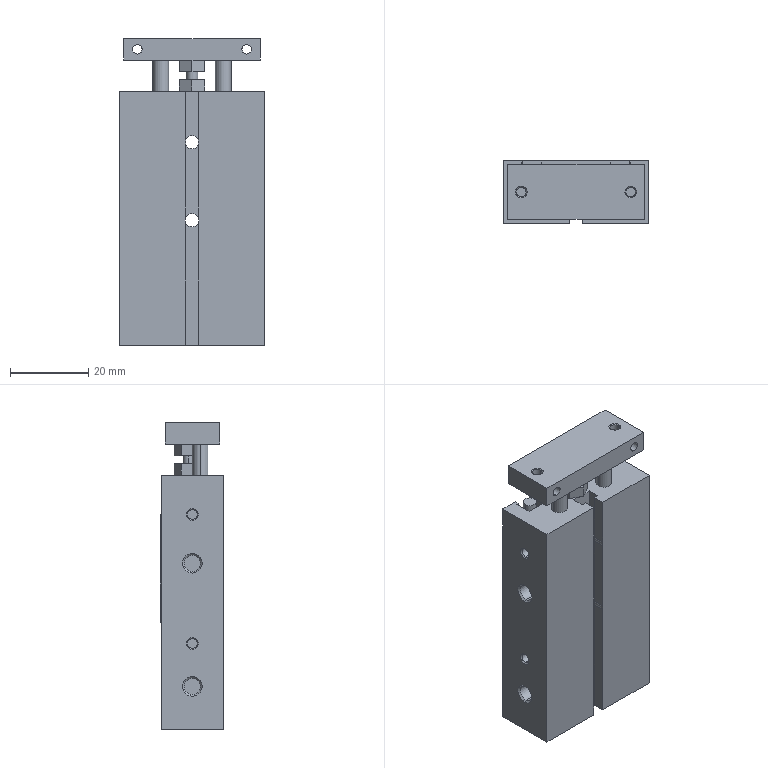Part | STEP file | Bag feed cylinder CXSM6-20-Z76L (0) | 1 solid | 166 faces | box 37 x 16.2 x 78.5 mm | volume 36756 mm3 | plane 86 | cylinder 56 | cone 24 | commonest cylinder face diameters 2.46 x24 3.4 x12 4.13 x8 3 x4 4 x4 6.5 x4